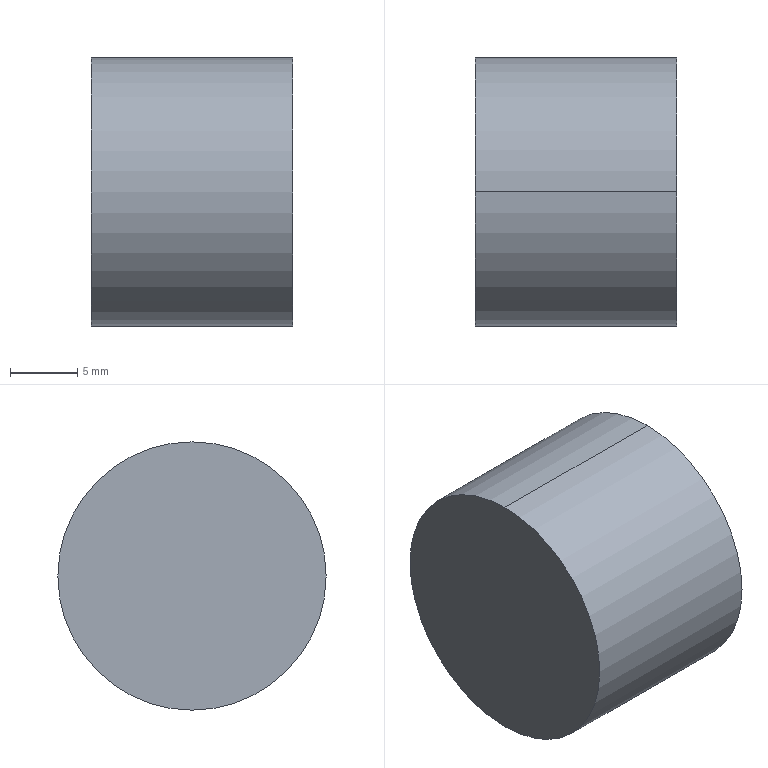Part | STEP file | Deraillieur Mounting spacer | 1 solid | 4 faces | box 15 x 20 x 20 mm | volume 4712 mm3 | cylinder 2 | plane 2 | commonest cylinder face diameters 20 x2
STEP:
#1=CARTESIAN_POINT('',(0.,0.,0.));
#2=DIRECTION('',(0.,0.,1.));
#3=DIRECTION('',(1.,0.,0.));
#4=AXIS2_PLACEMENT_3D('',#1,#2,#3);
#5=CARTESIAN_POINT('',(15.,0.,-10.));
#6=VERTEX_POINT('',#5);
#7=CARTESIAN_POINT('',(15.,0.,10.));
#8=VERTEX_POINT('',#7);
#9=CARTESIAN_POINT('',(15.,0.,0.));
#10=DIRECTION('',(1.,0.,0.));
#11=DIRECTION('',(0.,0.,-1.));
#12=AXIS2_PLACEMENT_3D('',#9,#10,#11);
#13=CIRCLE('',#12,10.);
#14=CARTESIAN_POINT('',(15.,0.,0.));
#15=DIRECTION('',(-1.,0.,0.));
#16=DIRECTION('',(0.,0.,1.));
#17=AXIS2_PLACEMENT_3D('',#14,#15,#16);
#18=CYLINDRICAL_SURFACE('',#17,10.);
#19=CARTESIAN_POINT('',(3.142,0.));
#20=DIRECTION('',(-1.,0.));
#21=VECTOR('',#20,1.);
#22=LINE('',#19,#21);
#23=(GEOMETRIC_REPRESENTATION_CONTEXT(2)PARAMETRIC_REPRESENTATION_CONTEXT()REPRESENTATION_CONTEXT('',''));
#24=DEFINITIONAL_REPRESENTATION('',(#22),#23);
#25=PCURVE('',#18,#24);
#26=CARTESIAN_POINT('',(15.,0.,0.));
#27=DIRECTION('',(1.,0.,0.));
#28=DIRECTION('',(0.,0.,-1.));
#29=AXIS2_PLACEMENT_3D('',#26,#27,#28);
#30=PLANE('',#29);
#31=CARTESIAN_POINT('',(0.,0.));
#32=DIRECTION('',(1.,0.));
#33=AXIS2_PLACEMENT_2D('',#31,#32);
#34=CIRCLE('',#33,10.);
#35=(GEOMETRIC_REPRESENTATION_CONTEXT(2)PARAMETRIC_REPRESENTATION_CONTEXT()REPRESENTATION_CONTEXT('',''));
#36=DEFINITIONAL_REPRESENTATION('',(#34),#35);
#37=PCURVE('',#30,#36);
#38=SURFACE_CURVE('',#13,(#25,#37),.PCURVE_S1.);
#39=EDGE_CURVE('',#6,#8,#38,.T.);
#40=ORIENTED_EDGE('',*,*,#39,.F.);
#41=CARTESIAN_POINT('',(0.,0.,-10.));
#42=VERTEX_POINT('',#41);
#43=CARTESIAN_POINT('',(15.,0.,-10.));
#44=DIRECTION('',(-1.,0.,0.));
#45=VECTOR('',#44,1.);
#46=LINE('',#43,#45);
#47=CARTESIAN_POINT('',(3.142,0.));
#48=DIRECTION('',(0.,1.));
#49=VECTOR('',#48,1.);
#50=LINE('',#47,#49);
#51=(GEOMETRIC_REPRESENTATION_CONTEXT(2)PARAMETRIC_REPRESENTATION_CONTEXT()REPRESENTATION_CONTEXT('',''));
#52=DEFINITIONAL_REPRESENTATION('',(#50),#51);
#53=PCURVE('',#18,#52);
#54=CARTESIAN_POINT('',(15.,0.,0.));
#55=DIRECTION('',(-1.,0.,0.));
#56=DIRECTION('',(0.,0.,1.));
#57=AXIS2_PLACEMENT_3D('',#54,#55,#56);
#58=CYLINDRICAL_SURFACE('',#57,10.);
#59=CARTESIAN_POINT('',(3.142,0.));
#60=DIRECTION('',(0.,1.));
#61=VECTOR('',#60,1.);
#62=LINE('',#59,#61);
#63=(GEOMETRIC_REPRESENTATION_CONTEXT(2)PARAMETRIC_REPRESENTATION_CONTEXT()REPRESENTATION_CONTEXT('',''));
#64=DEFINITIONAL_REPRESENTATION('',(#62),#63);
#65=PCURVE('',#58,#64);
#66=SURFACE_CURVE('',#46,(#53,#65),.PCURVE_S1.);
#67=EDGE_CURVE('',#6,#42,#66,.T.);
#68=ORIENTED_EDGE('',*,*,#67,.T.);
#69=CARTESIAN_POINT('',(0.,0.,10.));
#70=VERTEX_POINT('',#69);
#71=CARTESIAN_POINT('',(0.,0.,0.));
#72=DIRECTION('',(1.,0.,0.));
#73=DIRECTION('',(0.,0.,-1.));
#74=AXIS2_PLACEMENT_3D('',#71,#72,#73);
#75=CIRCLE('',#74,10.);
#76=CARTESIAN_POINT('',(3.142,15.));
#77=DIRECTION('',(-1.,0.));
#78=VECTOR('',#77,1.);
#79=LINE('',#76,#78);
#80=(GEOMETRIC_REPRESENTATION_CONTEXT(2)PARAMETRIC_REPRESENTATION_CONTEXT()REPRESENTATION_CONTEXT('',''));
#81=DEFINITIONAL_REPRESENTATION('',(#79),#80);
#82=PCURVE('',#18,#81);
#83=CARTESIAN_POINT('',(0.,0.,0.));
#84=DIRECTION('',(1.,0.,0.));
#85=DIRECTION('',(0.,0.,-1.));
#86=AXIS2_PLACEMENT_3D('',#83,#84,#85);
#87=PLANE('',#86);
#88=CARTESIAN_POINT('',(0.,0.));
#89=DIRECTION('',(1.,0.));
#90=AXIS2_PLACEMENT_2D('',#88,#89);
#91=CIRCLE('',#90,10.);
#92=(GEOMETRIC_REPRESENTATION_CONTEXT(2)PARAMETRIC_REPRESENTATION_CONTEXT()REPRESENTATION_CONTEXT('',''));
#93=DEFINITIONAL_REPRESENTATION('',(#91),#92);
#94=PCURVE('',#87,#93);
#95=SURFACE_CURVE('',#75,(#82,#94),.PCURVE_S1.);
#96=EDGE_CURVE('',#42,#70,#95,.T.);
#97=ORIENTED_EDGE('',*,*,#96,.T.);
#98=CARTESIAN_POINT('',(15.,0.,10.));
#99=DIRECTION('',(-1.,0.,0.));
#100=VECTOR('',#99,1.);
#101=LINE('',#98,#100);
#102=CARTESIAN_POINT('',(0.,0.));
#103=DIRECTION('',(0.,1.));
#104=VECTOR('',#103,1.);
#105=LINE('',#102,#104);
#106=(GEOMETRIC_REPRESENTATION_CONTEXT(2)PARAMETRIC_REPRESENTATION_CONTEXT()REPRESENTATION_CONTEXT('',''));
#107=DEFINITIONAL_REPRESENTATION('',(#105),#106);
#108=PCURVE('',#18,#107);
#109=CARTESIAN_POINT('',(6.283,0.));
#110=DIRECTION('',(0.,1.));
#111=VECTOR('',#110,1.);
#112=LINE('',#109,#111);
#113=(GEOMETRIC_REPRESENTATION_CONTEXT(2)PARAMETRIC_REPRESENTATION_CONTEXT()REPRESENTATION_CONTEXT('',''));
#114=DEFINITIONAL_REPRESENTATION('',(#112),#113);
#115=PCURVE('',#58,#114);
#116=SURFACE_CURVE('',#101,(#108,#115),.PCURVE_S1.);
#117=EDGE_CURVE('',#8,#70,#116,.T.);
#118=ORIENTED_EDGE('',*,*,#117,.F.);
#119=EDGE_LOOP('',(#40,#68,#97,#118));
#120=FACE_BOUND('',#119,.T.);
#121=ADVANCED_FACE('',(#120),#18,.T.);
#122=ORIENTED_EDGE('',*,*,#67,.F.);
#123=CARTESIAN_POINT('',(15.,0.,0.));
#124=DIRECTION('',(1.,0.,0.));
#125=DIRECTION('',(0.,0.,-1.));
#126=AXIS2_PLACEMENT_3D('',#123,#124,#125);
#127=CIRCLE('',#126,10.);
#128=CARTESIAN_POINT('',(9.425,0.));
#129=DIRECTION('',(-1.,0.));
#130=VECTOR('',#129,1.);
#131=LINE('',#128,#130);
#132=(GEOMETRIC_REPRESENTATION_CONTEXT(2)PARAMETRIC_REPRESENTATION_CONTEXT()REPRESENTATION_CONTEXT('',''));
#133=DEFINITIONAL_REPRESENTATION('',(#131),#132);
#134=PCURVE('',#58,#133);
#135=CARTESIAN_POINT('',(0.,0.));
#136=DIRECTION('',(1.,0.));
#137=AXIS2_PLACEMENT_2D('',#135,#136);
#138=CIRCLE('',#137,10.);
#139=(GEOMETRIC_REPRESENTATION_CONTEXT(2)PARAMETRIC_REPRESENTATION_CONTEXT()REPRESENTATION_CONTEXT('',''));
#140=DEFINITIONAL_REPRESENTATION('',(#138),#139);
#141=PCURVE('',#30,#140);
#142=SURFACE_CURVE('',#127,(#134,#141),.PCURVE_S1.);
#143=EDGE_CURVE('',#8,#6,#142,.T.);
#144=ORIENTED_EDGE('',*,*,#143,.F.);
#145=ORIENTED_EDGE('',*,*,#117,.T.);
#146=CARTESIAN_POINT('',(0.,0.,0.));
#147=DIRECTION('',(1.,0.,0.));
#148=DIRECTION('',(0.,0.,-1.));
#149=AXIS2_PLACEMENT_3D('',#146,#147,#148);
#150=CIRCLE('',#149,10.);
#151=CARTESIAN_POINT('',(9.425,15.));
#152=DIRECTION('',(-1.,0.));
#153=VECTOR('',#152,1.);
#154=LINE('',#151,#153);
#155=(GEOMETRIC_REPRESENTATION_CONTEXT(2)PARAMETRIC_REPRESENTATION_CONTEXT()REPRESENTATION_CONTEXT('',''));
#156=DEFINITIONAL_REPRESENTATION('',(#154),#155);
#157=PCURVE('',#58,#156);
#158=CARTESIAN_POINT('',(0.,0.));
#159=DIRECTION('',(1.,0.));
#160=AXIS2_PLACEMENT_2D('',#158,#159);
#161=CIRCLE('',#160,10.);
#162=(GEOMETRIC_REPRESENTATION_CONTEXT(2)PARAMETRIC_REPRESENTATION_CONTEXT()REPRESENTATION_CONTEXT('',''));
#163=DEFINITIONAL_REPRESENTATION('',(#161),#162);
#164=PCURVE('',#87,#163);
#165=SURFACE_CURVE('',#150,(#157,#164),.PCURVE_S1.);
#166=EDGE_CURVE('',#70,#42,#165,.T.);
#167=ORIENTED_EDGE('',*,*,#166,.T.);
#168=EDGE_LOOP('',(#122,#144,#145,#167));
#169=FACE_BOUND('',#168,.T.);
#170=ADVANCED_FACE('',(#169),#58,.T.);
#171=ORIENTED_EDGE('',*,*,#143,.T.);
#172=ORIENTED_EDGE('',*,*,#39,.T.);
#173=EDGE_LOOP('',(#171,#172));
#174=FACE_BOUND('',#173,.T.);
#175=ADVANCED_FACE('',(#174),#30,.T.);
#176=ORIENTED_EDGE('',*,*,#166,.F.);
#177=ORIENTED_EDGE('',*,*,#96,.F.);
#178=EDGE_LOOP('',(#176,#177));
#179=FACE_BOUND('',#178,.T.);
#180=ADVANCED_FACE('',(#179),#87,.F.);
#181=CLOSED_SHELL('',(#121,#170,#175,#180));
#182=MANIFOLD_SOLID_BREP('',#181);
#183=(LENGTH_UNIT()NAMED_UNIT(*)SI_UNIT(.MILLI.,.METRE.));
#184=UNCERTAINTY_MEASURE_WITH_UNIT(LENGTH_MEASURE(0.0000001),#183,'','');
#185=(NAMED_UNIT(*)PLANE_ANGLE_UNIT()SI_UNIT($,.RADIAN.));
#186=(NAMED_UNIT(*)SI_UNIT($,.STERADIAN.)SOLID_ANGLE_UNIT());
#187=(GEOMETRIC_REPRESENTATION_CONTEXT(3)GLOBAL_UNCERTAINTY_ASSIGNED_CONTEXT((#184))GLOBAL_UNIT_ASSIGNED_CONTEXT((#183,#185,#186))REPRESENTATION_CONTEXT('',''));
#188=ADVANCED_BREP_SHAPE_REPRESENTATION('',(#4,#182),#187);